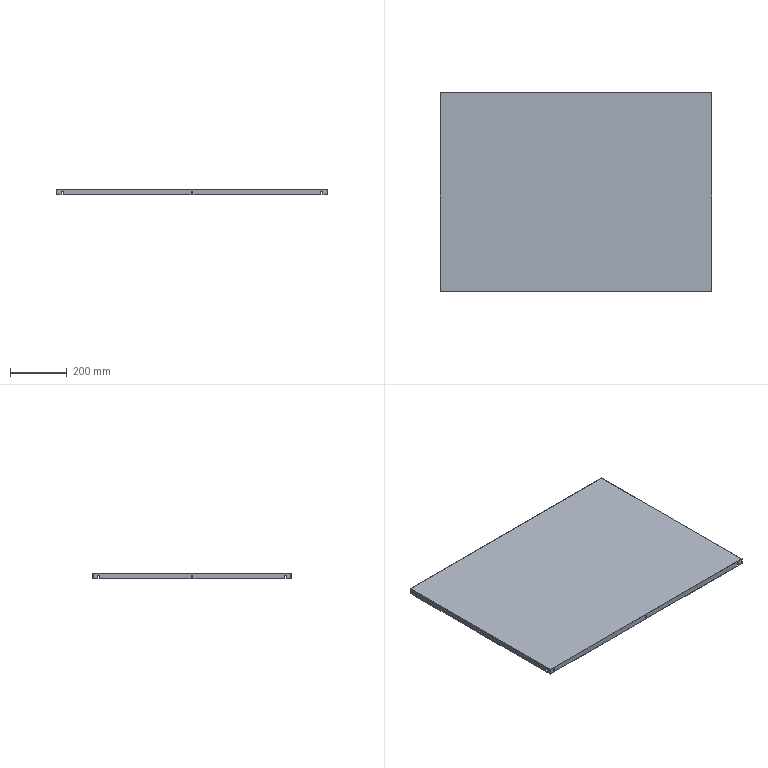Part | STEP file | PN_0009 | 1 solid | 64 faces | box 955 x 698 x 20 mm | volume 728257 mm3 | plane 46 | cylinder 18 | commonest cylinder face diameters 7 x18